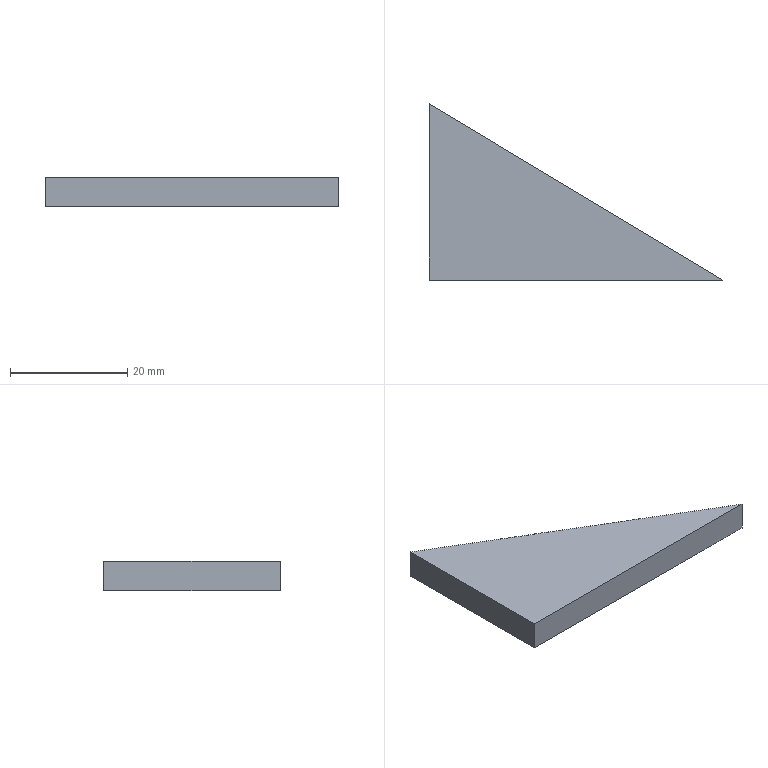Part | SolidWorks | features Extrusion 1 | 1 solid | 5 faces | box 50 x 30 x 5 mm | volume 3750 mm3 | plane 5
STEP:
#1=CARTESIAN_POINT('',(0.,0.,0.));
#2=VERTEX_POINT('',#1);
#3=CARTESIAN_POINT('',(50.,0.,0.));
#4=VERTEX_POINT('',#3);
#5=CARTESIAN_POINT('',(0.,0.,0.));
#6=DIRECTION('',(1.,0.,0.));
#7=VECTOR('',#6,1000.);
#8=LINE('',#5,#7);
#9=EDGE_CURVE('',#2,#4,#8,.T.);
#10=ORIENTED_EDGE('',*,*,#9,.T.);
#11=CARTESIAN_POINT('',(50.,0.,5.));
#12=VERTEX_POINT('',#11);
#13=CARTESIAN_POINT('',(50.,0.,5.));
#14=DIRECTION('',(0.,0.,-1.));
#15=VECTOR('',#14,1000.);
#16=LINE('',#13,#15);
#17=EDGE_CURVE('',#12,#4,#16,.T.);
#18=ORIENTED_EDGE('',*,*,#17,.F.);
#19=CARTESIAN_POINT('',(0.,0.,5.));
#20=VERTEX_POINT('',#19);
#21=CARTESIAN_POINT('',(0.,0.,5.));
#22=DIRECTION('',(1.,0.,0.));
#23=VECTOR('',#22,1000.);
#24=LINE('',#21,#23);
#25=EDGE_CURVE('',#20,#12,#24,.T.);
#26=ORIENTED_EDGE('',*,*,#25,.F.);
#27=CARTESIAN_POINT('',(0.,0.,5.));
#28=DIRECTION('',(0.,0.,-1.));
#29=VECTOR('',#28,1000.);
#30=LINE('',#27,#29);
#31=EDGE_CURVE('',#20,#2,#30,.T.);
#32=ORIENTED_EDGE('',*,*,#31,.T.);
#33=EDGE_LOOP('',(#10,#18,#26,#32));
#34=FACE_OUTER_BOUND('',#33,.T.);
#35=CARTESIAN_POINT('',(0.,0.,5.));
#36=DIRECTION('',(0.,1.,0.));
#37=DIRECTION('',(0.,0.,1.));
#38=AXIS2_PLACEMENT_3D('',#35,#36,#37);
#39=PLANE('',#38);
#40=ADVANCED_FACE('',(#34),#39,.F.);
#41=CARTESIAN_POINT('',(0.,30.,0.));
#42=VERTEX_POINT('',#41);
#43=CARTESIAN_POINT('',(50.,0.,0.));
#44=DIRECTION('',(-0.8575,0.5145,0.));
#45=VECTOR('',#44,1000.);
#46=LINE('',#43,#45);
#47=EDGE_CURVE('',#4,#42,#46,.T.);
#48=ORIENTED_EDGE('',*,*,#47,.T.);
#49=CARTESIAN_POINT('',(0.,30.,5.));
#50=VERTEX_POINT('',#49);
#51=CARTESIAN_POINT('',(0.,30.,5.));
#52=DIRECTION('',(0.,0.,-1.));
#53=VECTOR('',#52,1000.);
#54=LINE('',#51,#53);
#55=EDGE_CURVE('',#50,#42,#54,.T.);
#56=ORIENTED_EDGE('',*,*,#55,.F.);
#57=CARTESIAN_POINT('',(50.,0.,5.));
#58=DIRECTION('',(-0.8575,0.5145,0.));
#59=VECTOR('',#58,1000.);
#60=LINE('',#57,#59);
#61=EDGE_CURVE('',#12,#50,#60,.T.);
#62=ORIENTED_EDGE('',*,*,#61,.F.);
#63=ORIENTED_EDGE('',*,*,#17,.T.);
#64=EDGE_LOOP('',(#48,#56,#62,#63));
#65=FACE_OUTER_BOUND('',#64,.T.);
#66=CARTESIAN_POINT('',(50.,0.,5.));
#67=DIRECTION('',(-0.5145,-0.8575,0.));
#68=DIRECTION('',(0.8575,-0.5145,0.));
#69=AXIS2_PLACEMENT_3D('',#66,#67,#68);
#70=PLANE('',#69);
#71=ADVANCED_FACE('',(#65),#70,.F.);
#72=CARTESIAN_POINT('',(0.,0.,0.));
#73=DIRECTION('',(0.,-1.,0.));
#74=VECTOR('',#73,1000.);
#75=LINE('',#72,#74);
#76=EDGE_CURVE('',#42,#2,#75,.T.);
#77=ORIENTED_EDGE('',*,*,#76,.T.);
#78=ORIENTED_EDGE('',*,*,#31,.F.);
#79=CARTESIAN_POINT('',(0.,0.,5.));
#80=DIRECTION('',(0.,-1.,0.));
#81=VECTOR('',#80,1000.);
#82=LINE('',#79,#81);
#83=EDGE_CURVE('',#50,#20,#82,.T.);
#84=ORIENTED_EDGE('',*,*,#83,.F.);
#85=ORIENTED_EDGE('',*,*,#55,.T.);
#86=EDGE_LOOP('',(#77,#78,#84,#85));
#87=FACE_OUTER_BOUND('',#86,.T.);
#88=CARTESIAN_POINT('',(0.,0.,5.));
#89=DIRECTION('',(1.,0.,0.));
#90=DIRECTION('',(0.,0.,-1.));
#91=AXIS2_PLACEMENT_3D('',#88,#89,#90);
#92=PLANE('',#91);
#93=ADVANCED_FACE('',(#87),#92,.F.);
#94=ORIENTED_EDGE('',*,*,#25,.T.);
#95=ORIENTED_EDGE('',*,*,#61,.T.);
#96=ORIENTED_EDGE('',*,*,#83,.T.);
#97=EDGE_LOOP('',(#94,#95,#96));
#98=FACE_OUTER_BOUND('',#97,.T.);
#99=CARTESIAN_POINT('',(0.,0.,5.));
#100=DIRECTION('',(0.,0.,1.));
#101=DIRECTION('',(1.,0.,0.));
#102=AXIS2_PLACEMENT_3D('',#99,#100,#101);
#103=PLANE('',#102);
#104=ADVANCED_FACE('',(#98),#103,.T.);
#105=ORIENTED_EDGE('',*,*,#9,.F.);
#106=ORIENTED_EDGE('',*,*,#76,.F.);
#107=ORIENTED_EDGE('',*,*,#47,.F.);
#108=EDGE_LOOP('',(#105,#106,#107));
#109=FACE_OUTER_BOUND('',#108,.T.);
#110=CARTESIAN_POINT('',(0.,0.,0.));
#111=DIRECTION('',(0.,0.,1.));
#112=DIRECTION('',(1.,0.,0.));
#113=AXIS2_PLACEMENT_3D('',#110,#111,#112);
#114=PLANE('',#113);
#115=ADVANCED_FACE('',(#109),#114,.F.);
#116=CLOSED_SHELL('',(#40,#71,#93,#104,#115));
#117=MANIFOLD_SOLID_BREP('',#116);
#118=CARTESIAN_POINT('',(0.,0.,0.));
#119=DIRECTION('',(0.,0.,1.));
#120=DIRECTION('',(1.,0.,0.));
#121=AXIS2_PLACEMENT_3D('',#118,#119,#120);
#122=(LENGTH_UNIT()NAMED_UNIT(*)SI_UNIT(.MILLI.,.METRE.));
#123=UNCERTAINTY_MEASURE_WITH_UNIT(LENGTH_MEASURE(0.00001),#122,'','');
#124=(NAMED_UNIT(*)PLANE_ANGLE_UNIT()SI_UNIT($,.RADIAN.));
#125=(NAMED_UNIT(*)SI_UNIT($,.STERADIAN.)SOLID_ANGLE_UNIT());
#126=(GEOMETRIC_REPRESENTATION_CONTEXT(3)GLOBAL_UNCERTAINTY_ASSIGNED_CONTEXT((#123))GLOBAL_UNIT_ASSIGNED_CONTEXT((#122,#124,#125))REPRESENTATION_CONTEXT('',''));
#127=ADVANCED_BREP_SHAPE_REPRESENTATION('',(#117,#121),#126);